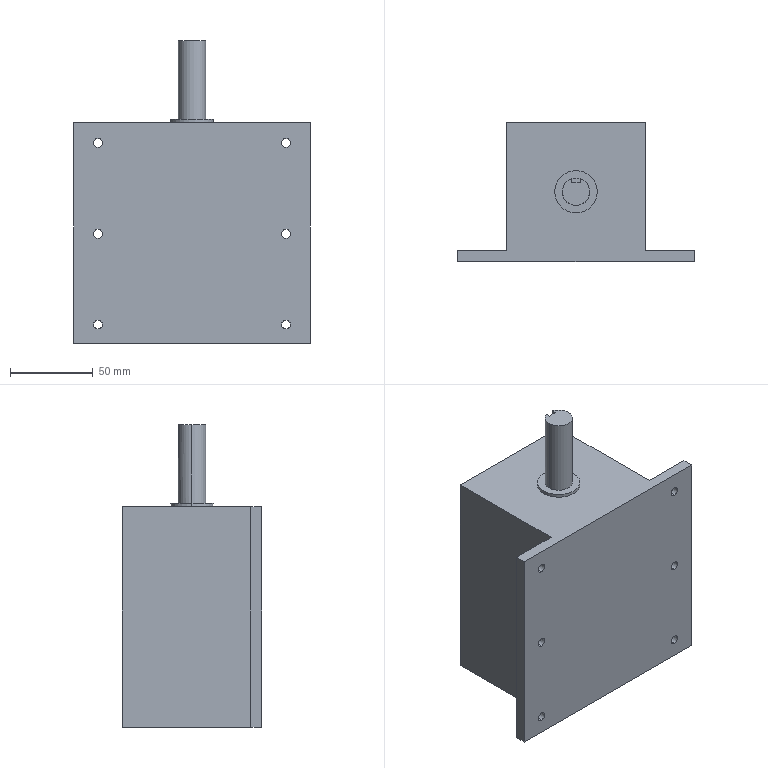Part | SolidWorks | features BaseBody 1, ICE 1 | 1 solid | 32 faces | box 143.331 x 84.235 x 183.45 mm | volume 1010969 mm3 | cylinder 16 | plane 16 | commonest cylinder face diameters 5.365 x12 16.643 x2 25.738 x2
STEP:
#1=CARTESIAN_POINT('',(-135.383,-355.58,-9.625));
#2=VERTEX_POINT('',#1);
#3=CARTESIAN_POINT('',(-135.383,-355.58,-14.99));
#4=VERTEX_POINT('',#3);
#5=CARTESIAN_POINT('',(-135.383,-355.58,-12.308));
#6=DIRECTION('',(0.,-1.,0.));
#7=DIRECTION('',(0.,0.,-1.));
#8=AXIS2_PLACEMENT_3D('',#5,#6,#7);
#9=CIRCLE('',#8,2.683);
#10=EDGE_CURVE('',#2,#4,#9,.T.);
#11=ORIENTED_EDGE('',*,*,#10,.F.);
#12=CARTESIAN_POINT('',(-135.383,-362.11,-9.625));
#13=VERTEX_POINT('',#12);
#14=CARTESIAN_POINT('',(-135.383,-355.58,-9.625));
#15=DIRECTION('',(0.,-1.,0.));
#16=VECTOR('',#15,1000.);
#17=LINE('',#14,#16);
#18=EDGE_CURVE('',#2,#13,#17,.T.);
#19=ORIENTED_EDGE('',*,*,#18,.T.);
#20=CARTESIAN_POINT('',(-135.383,-362.11,-14.99));
#21=VERTEX_POINT('',#20);
#22=CARTESIAN_POINT('',(-135.383,-362.11,-12.308));
#23=DIRECTION('',(0.,1.,0.));
#24=DIRECTION('',(0.,0.,-1.));
#25=AXIS2_PLACEMENT_3D('',#22,#23,#24);
#26=CIRCLE('',#25,2.683);
#27=EDGE_CURVE('',#21,#13,#26,.T.);
#28=ORIENTED_EDGE('',*,*,#27,.F.);
#29=CARTESIAN_POINT('',(-135.383,-355.58,-14.99));
#30=DIRECTION('',(0.,-1.,0.));
#31=VECTOR('',#30,1000.);
#32=LINE('',#29,#31);
#33=EDGE_CURVE('',#4,#21,#32,.T.);
#34=ORIENTED_EDGE('',*,*,#33,.F.);
#35=EDGE_LOOP('',(#11,#19,#28,#34));
#36=FACE_OUTER_BOUND('',#35,.T.);
#37=CARTESIAN_POINT('',(-135.383,-355.58,-12.308));
#38=DIRECTION('',(0.,-1.,0.));
#39=DIRECTION('',(0.,0.,-1.));
#40=AXIS2_PLACEMENT_3D('',#37,#38,#39);
#41=CYLINDRICAL_SURFACE('',#40,2.683);
#42=ADVANCED_FACE('',(#36),#41,.F.);
#43=CARTESIAN_POINT('',(-135.383,-355.58,-64.625));
#44=VERTEX_POINT('',#43);
#45=CARTESIAN_POINT('',(-135.383,-355.58,-69.99));
#46=VERTEX_POINT('',#45);
#47=CARTESIAN_POINT('',(-135.383,-355.58,-67.308));
#48=DIRECTION('',(0.,-1.,0.));
#49=DIRECTION('',(0.,0.,-1.));
#50=AXIS2_PLACEMENT_3D('',#47,#48,#49);
#51=CIRCLE('',#50,2.683);
#52=EDGE_CURVE('',#44,#46,#51,.T.);
#53=ORIENTED_EDGE('',*,*,#52,.F.);
#54=CARTESIAN_POINT('',(-135.383,-362.11,-64.625));
#55=VERTEX_POINT('',#54);
#56=CARTESIAN_POINT('',(-135.383,-355.58,-64.625));
#57=DIRECTION('',(0.,-1.,0.));
#58=VECTOR('',#57,1000.);
#59=LINE('',#56,#58);
#60=EDGE_CURVE('',#44,#55,#59,.T.);
#61=ORIENTED_EDGE('',*,*,#60,.T.);
#62=CARTESIAN_POINT('',(-135.383,-362.11,-69.99));
#63=VERTEX_POINT('',#62);
#64=CARTESIAN_POINT('',(-135.383,-362.11,-67.308));
#65=DIRECTION('',(0.,1.,0.));
#66=DIRECTION('',(0.,0.,-1.));
#67=AXIS2_PLACEMENT_3D('',#64,#65,#66);
#68=CIRCLE('',#67,2.683);
#69=EDGE_CURVE('',#63,#55,#68,.T.);
#70=ORIENTED_EDGE('',*,*,#69,.F.);
#71=CARTESIAN_POINT('',(-135.383,-355.58,-69.99));
#72=DIRECTION('',(0.,-1.,0.));
#73=VECTOR('',#72,1000.);
#74=LINE('',#71,#73);
#75=EDGE_CURVE('',#46,#63,#74,.T.);
#76=ORIENTED_EDGE('',*,*,#75,.F.);
#77=EDGE_LOOP('',(#53,#61,#70,#76));
#78=FACE_OUTER_BOUND('',#77,.T.);
#79=CARTESIAN_POINT('',(-135.383,-355.58,-67.308));
#80=DIRECTION('',(0.,-1.,0.));
#81=DIRECTION('',(0.,0.,-1.));
#82=AXIS2_PLACEMENT_3D('',#79,#80,#81);
#83=CYLINDRICAL_SURFACE('',#82,2.683);
#84=ADVANCED_FACE('',(#78),#83,.F.);
#85=CARTESIAN_POINT('',(-135.383,-355.58,-119.625));
#86=VERTEX_POINT('',#85);
#87=CARTESIAN_POINT('',(-135.383,-355.58,-124.99));
#88=VERTEX_POINT('',#87);
#89=CARTESIAN_POINT('',(-135.383,-355.58,-122.308));
#90=DIRECTION('',(0.,-1.,0.));
#91=DIRECTION('',(0.,0.,-1.));
#92=AXIS2_PLACEMENT_3D('',#89,#90,#91);
#93=CIRCLE('',#92,2.683);
#94=EDGE_CURVE('',#86,#88,#93,.T.);
#95=ORIENTED_EDGE('',*,*,#94,.F.);
#96=CARTESIAN_POINT('',(-135.383,-362.11,-119.625));
#97=VERTEX_POINT('',#96);
#98=CARTESIAN_POINT('',(-135.383,-355.58,-119.625));
#99=DIRECTION('',(0.,-1.,0.));
#100=VECTOR('',#99,1000.);
#101=LINE('',#98,#100);
#102=EDGE_CURVE('',#86,#97,#101,.T.);
#103=ORIENTED_EDGE('',*,*,#102,.T.);
#104=CARTESIAN_POINT('',(-135.383,-362.11,-124.99));
#105=VERTEX_POINT('',#104);
#106=CARTESIAN_POINT('',(-135.383,-362.11,-122.308));
#107=DIRECTION('',(0.,1.,0.));
#108=DIRECTION('',(0.,0.,-1.));
#109=AXIS2_PLACEMENT_3D('',#106,#107,#108);
#110=CIRCLE('',#109,2.683);
#111=EDGE_CURVE('',#105,#97,#110,.T.);
#112=ORIENTED_EDGE('',*,*,#111,.F.);
#113=CARTESIAN_POINT('',(-135.383,-355.58,-124.99));
#114=DIRECTION('',(0.,-1.,0.));
#115=VECTOR('',#114,1000.);
#116=LINE('',#113,#115);
#117=EDGE_CURVE('',#88,#105,#116,.T.);
#118=ORIENTED_EDGE('',*,*,#117,.F.);
#119=EDGE_LOOP('',(#95,#103,#112,#118));
#120=FACE_OUTER_BOUND('',#119,.T.);
#121=CARTESIAN_POINT('',(-135.383,-355.58,-122.308));
#122=DIRECTION('',(0.,-1.,0.));
#123=DIRECTION('',(0.,0.,-1.));
#124=AXIS2_PLACEMENT_3D('',#121,#122,#123);
#125=CYLINDRICAL_SURFACE('',#124,2.683);
#126=ADVANCED_FACE('',(#120),#125,.F.);
#127=CARTESIAN_POINT('',(-21.6,-355.58,-9.625));
#128=VERTEX_POINT('',#127);
#129=CARTESIAN_POINT('',(-21.6,-355.58,-14.99));
#130=VERTEX_POINT('',#129);
#131=CARTESIAN_POINT('',(-21.6,-355.58,-12.308));
#132=DIRECTION('',(0.,-1.,0.));
#133=DIRECTION('',(0.,0.,-1.));
#134=AXIS2_PLACEMENT_3D('',#131,#132,#133);
#135=CIRCLE('',#134,2.683);
#136=EDGE_CURVE('',#128,#130,#135,.T.);
#137=ORIENTED_EDGE('',*,*,#136,.F.);
#138=CARTESIAN_POINT('',(-21.6,-362.11,-9.625));
#139=VERTEX_POINT('',#138);
#140=CARTESIAN_POINT('',(-21.6,-355.58,-9.625));
#141=DIRECTION('',(0.,-1.,0.));
#142=VECTOR('',#141,1000.);
#143=LINE('',#140,#142);
#144=EDGE_CURVE('',#128,#139,#143,.T.);
#145=ORIENTED_EDGE('',*,*,#144,.T.);
#146=CARTESIAN_POINT('',(-21.6,-362.11,-14.99));
#147=VERTEX_POINT('',#146);
#148=CARTESIAN_POINT('',(-21.6,-362.11,-12.308));
#149=DIRECTION('',(0.,1.,0.));
#150=DIRECTION('',(0.,0.,-1.));
#151=AXIS2_PLACEMENT_3D('',#148,#149,#150);
#152=CIRCLE('',#151,2.683);
#153=EDGE_CURVE('',#147,#139,#152,.T.);
#154=ORIENTED_EDGE('',*,*,#153,.F.);
#155=CARTESIAN_POINT('',(-21.6,-355.58,-14.99));
#156=DIRECTION('',(0.,-1.,0.));
#157=VECTOR('',#156,1000.);
#158=LINE('',#155,#157);
#159=EDGE_CURVE('',#130,#147,#158,.T.);
#160=ORIENTED_EDGE('',*,*,#159,.F.);
#161=EDGE_LOOP('',(#137,#145,#154,#160));
#162=FACE_OUTER_BOUND('',#161,.T.);
#163=CARTESIAN_POINT('',(-21.6,-355.58,-12.308));
#164=DIRECTION('',(0.,-1.,0.));
#165=DIRECTION('',(0.,0.,-1.));
#166=AXIS2_PLACEMENT_3D('',#163,#164,#165);
#167=CYLINDRICAL_SURFACE('',#166,2.683);
#168=ADVANCED_FACE('',(#162),#167,.F.);
#169=CARTESIAN_POINT('',(-21.6,-355.58,-64.625));
#170=VERTEX_POINT('',#169);
#171=CARTESIAN_POINT('',(-21.6,-355.58,-69.99));
#172=VERTEX_POINT('',#171);
#173=CARTESIAN_POINT('',(-21.6,-355.58,-67.308));
#174=DIRECTION('',(0.,-1.,0.));
#175=DIRECTION('',(0.,0.,-1.));
#176=AXIS2_PLACEMENT_3D('',#173,#174,#175);
#177=CIRCLE('',#176,2.683);
#178=EDGE_CURVE('',#170,#172,#177,.T.);
#179=ORIENTED_EDGE('',*,*,#178,.F.);
#180=CARTESIAN_POINT('',(-21.6,-362.11,-64.625));
#181=VERTEX_POINT('',#180);
#182=CARTESIAN_POINT('',(-21.6,-355.58,-64.625));
#183=DIRECTION('',(0.,-1.,0.));
#184=VECTOR('',#183,1000.);
#185=LINE('',#182,#184);
#186=EDGE_CURVE('',#170,#181,#185,.T.);
#187=ORIENTED_EDGE('',*,*,#186,.T.);
#188=CARTESIAN_POINT('',(-21.6,-362.11,-69.99));
#189=VERTEX_POINT('',#188);
#190=CARTESIAN_POINT('',(-21.6,-362.11,-67.308));
#191=DIRECTION('',(0.,1.,0.));
#192=DIRECTION('',(0.,0.,-1.));
#193=AXIS2_PLACEMENT_3D('',#190,#191,#192);
#194=CIRCLE('',#193,2.683);
#195=EDGE_CURVE('',#189,#181,#194,.T.);
#196=ORIENTED_EDGE('',*,*,#195,.F.);
#197=CARTESIAN_POINT('',(-21.6,-355.58,-69.99));
#198=DIRECTION('',(0.,-1.,0.));
#199=VECTOR('',#198,1000.);
#200=LINE('',#197,#199);
#201=EDGE_CURVE('',#172,#189,#200,.T.);
#202=ORIENTED_EDGE('',*,*,#201,.F.);
#203=EDGE_LOOP('',(#179,#187,#196,#202));
#204=FACE_OUTER_BOUND('',#203,.T.);
#205=CARTESIAN_POINT('',(-21.6,-355.58,-67.308));
#206=DIRECTION('',(0.,-1.,0.));
#207=DIRECTION('',(0.,0.,-1.));
#208=AXIS2_PLACEMENT_3D('',#205,#206,#207);
#209=CYLINDRICAL_SURFACE('',#208,2.683);
#210=ADVANCED_FACE('',(#204),#209,.F.);
#211=CARTESIAN_POINT('',(-21.6,-355.58,-119.625));
#212=VERTEX_POINT('',#211);
#213=CARTESIAN_POINT('',(-21.6,-355.58,-124.99));
#214=VERTEX_POINT('',#213);
#215=CARTESIAN_POINT('',(-21.6,-355.58,-122.308));
#216=DIRECTION('',(0.,-1.,0.));
#217=DIRECTION('',(0.,0.,-1.));
#218=AXIS2_PLACEMENT_3D('',#215,#216,#217);
#219=CIRCLE('',#218,2.683);
#220=EDGE_CURVE('',#212,#214,#219,.T.);
#221=ORIENTED_EDGE('',*,*,#220,.F.);
#222=CARTESIAN_POINT('',(-21.6,-362.11,-119.625));
#223=VERTEX_POINT('',#222);
#224=CARTESIAN_POINT('',(-21.6,-355.58,-119.625));
#225=DIRECTION('',(0.,-1.,0.));
#226=VECTOR('',#225,1000.);
#227=LINE('',#224,#226);
#228=EDGE_CURVE('',#212,#223,#227,.T.);
#229=ORIENTED_EDGE('',*,*,#228,.T.);
#230=CARTESIAN_POINT('',(-21.6,-362.11,-124.99));
#231=VERTEX_POINT('',#230);
#232=CARTESIAN_POINT('',(-21.6,-362.11,-122.308));
#233=DIRECTION('',(0.,1.,0.));
#234=DIRECTION('',(0.,0.,-1.));
#235=AXIS2_PLACEMENT_3D('',#232,#233,#234);
#236=CIRCLE('',#235,2.683);
#237=EDGE_CURVE('',#231,#223,#236,.T.);
#238=ORIENTED_EDGE('',*,*,#237,.F.);
#239=CARTESIAN_POINT('',(-21.6,-355.58,-124.99));
#240=DIRECTION('',(0.,-1.,0.));
#241=VECTOR('',#240,1000.);
#242=LINE('',#239,#241);
#243=EDGE_CURVE('',#214,#231,#242,.T.);
#244=ORIENTED_EDGE('',*,*,#243,.F.);
#245=EDGE_LOOP('',(#221,#229,#238,#244));
#246=FACE_OUTER_BOUND('',#245,.T.);
#247=CARTESIAN_POINT('',(-21.6,-355.58,-122.308));
#248=DIRECTION('',(0.,-1.,0.));
#249=DIRECTION('',(0.,0.,-1.));
#250=AXIS2_PLACEMENT_3D('',#247,#248,#249);
#251=CYLINDRICAL_SURFACE('',#250,2.683);
#252=ADVANCED_FACE('',(#246),#251,.F.);
#253=CARTESIAN_POINT('',(-65.623,-319.993,0.));
#254=VERTEX_POINT('',#253);
#255=CARTESIAN_POINT('',(-91.361,-319.993,0.));
#256=VERTEX_POINT('',#255);
#257=CARTESIAN_POINT('',(-78.492,-319.993,0.));
#258=DIRECTION('',(0.,0.,1.));
#259=DIRECTION('',(1.,0.,0.));
#260=AXIS2_PLACEMENT_3D('',#257,#258,#259);
#261=CIRCLE('',#260,12.869);
#262=EDGE_CURVE('',#254,#256,#261,.T.);
#263=ORIENTED_EDGE('',*,*,#262,.T.);
#264=CARTESIAN_POINT('',(-91.361,-319.993,2.));
#265=VERTEX_POINT('',#264);
#266=CARTESIAN_POINT('',(-91.361,-319.993,0.));
#267=DIRECTION('',(0.,0.,1.));
#268=VECTOR('',#267,1000.);
#269=LINE('',#266,#268);
#270=EDGE_CURVE('',#256,#265,#269,.T.);
#271=ORIENTED_EDGE('',*,*,#270,.T.);
#272=CARTESIAN_POINT('',(-65.623,-319.993,2.));
#273=VERTEX_POINT('',#272);
#274=CARTESIAN_POINT('',(-78.492,-319.993,2.));
#275=DIRECTION('',(0.,0.,-1.));
#276=DIRECTION('',(1.,0.,0.));
#277=AXIS2_PLACEMENT_3D('',#274,#275,#276);
#278=CIRCLE('',#277,12.869);
#279=EDGE_CURVE('',#265,#273,#278,.T.);
#280=ORIENTED_EDGE('',*,*,#279,.T.);
#281=CARTESIAN_POINT('',(-65.623,-319.993,0.));
#282=DIRECTION('',(0.,0.,1.));
#283=VECTOR('',#282,1000.);
#284=LINE('',#281,#283);
#285=EDGE_CURVE('',#254,#273,#284,.T.);
#286=ORIENTED_EDGE('',*,*,#285,.F.);
#287=EDGE_LOOP('',(#263,#271,#280,#286));
#288=FACE_OUTER_BOUND('',#287,.T.);
#289=CARTESIAN_POINT('',(-78.492,-319.993,0.));
#290=DIRECTION('',(0.,0.,1.));
#291=DIRECTION('',(1.,0.,0.));
#292=AXIS2_PLACEMENT_3D('',#289,#290,#291);
#293=CYLINDRICAL_SURFACE('',#292,12.869);
#294=ADVANCED_FACE('',(#288),#293,.T.);
#295=CARTESIAN_POINT('',(-70.17,-319.993,2.));
#296=VERTEX_POINT('',#295);
#297=CARTESIAN_POINT('',(-86.814,-319.993,2.));
#298=VERTEX_POINT('',#297);
#299=CARTESIAN_POINT('',(-78.492,-319.993,2.));
#300=DIRECTION('',(0.,0.,1.));
#301=DIRECTION('',(1.,0.,0.));
#302=AXIS2_PLACEMENT_3D('',#299,#300,#301);
#303=CIRCLE('',#302,8.322);
#304=EDGE_CURVE('',#296,#298,#303,.T.);
#305=ORIENTED_EDGE('',*,*,#304,.T.);
#306=CARTESIAN_POINT('',(-86.814,-319.993,49.688));
#307=VERTEX_POINT('',#306);
#308=CARTESIAN_POINT('',(-86.814,-319.993,0.));
#309=DIRECTION('',(0.,0.,1.));
#310=VECTOR('',#309,1000.);
#311=LINE('',#308,#310);
#312=EDGE_CURVE('',#298,#307,#311,.T.);
#313=ORIENTED_EDGE('',*,*,#312,.T.);
#314=CARTESIAN_POINT('',(-80.992,-312.055,49.688));
#315=VERTEX_POINT('',#314);
#316=CARTESIAN_POINT('',(-78.492,-319.993,49.688));
#317=DIRECTION('',(0.,0.,-1.));
#318=DIRECTION('',(1.,0.,0.));
#319=AXIS2_PLACEMENT_3D('',#316,#317,#318);
#320=CIRCLE('',#319,8.322);
#321=EDGE_CURVE('',#307,#315,#320,.T.);
#322=ORIENTED_EDGE('',*,*,#321,.T.);
#323=CARTESIAN_POINT('',(-80.992,-312.055,29.688));
#324=VERTEX_POINT('',#323);
#325=CARTESIAN_POINT('',(-80.992,-312.055,0.));
#326=DIRECTION('',(0.,0.,1.));
#327=VECTOR('',#326,1000.);
#328=LINE('',#325,#327);
#329=EDGE_CURVE('',#324,#315,#328,.T.);
#330=ORIENTED_EDGE('',*,*,#329,.F.);
#331=CARTESIAN_POINT('',(-75.992,-312.055,29.688));
#332=VERTEX_POINT('',#331);
#333=CARTESIAN_POINT('',(-78.492,-319.993,29.688));
#334=DIRECTION('',(0.,0.,-1.));
#335=DIRECTION('',(1.,0.,0.));
#336=AXIS2_PLACEMENT_3D('',#333,#334,#335);
#337=CIRCLE('',#336,8.322);
#338=EDGE_CURVE('',#324,#332,#337,.T.);
#339=ORIENTED_EDGE('',*,*,#338,.T.);
#340=CARTESIAN_POINT('',(-75.992,-312.055,49.688));
#341=VERTEX_POINT('',#340);
#342=CARTESIAN_POINT('',(-75.992,-312.055,0.));
#343=DIRECTION('',(0.,0.,-1.));
#344=VECTOR('',#343,1000.);
#345=LINE('',#342,#344);
#346=EDGE_CURVE('',#341,#332,#345,.T.);
#347=ORIENTED_EDGE('',*,*,#346,.F.);
#348=CARTESIAN_POINT('',(-70.17,-319.993,49.688));
#349=VERTEX_POINT('',#348);
#350=CARTESIAN_POINT('',(-78.492,-319.993,49.688));
#351=DIRECTION('',(0.,0.,-1.));
#352=DIRECTION('',(1.,0.,0.));
#353=AXIS2_PLACEMENT_3D('',#350,#351,#352);
#354=CIRCLE('',#353,8.322);
#355=EDGE_CURVE('',#341,#349,#354,.T.);
#356=ORIENTED_EDGE('',*,*,#355,.T.);
#357=CARTESIAN_POINT('',(-70.17,-319.993,0.));
#358=DIRECTION('',(0.,0.,1.));
#359=VECTOR('',#358,1000.);
#360=LINE('',#357,#359);
#361=EDGE_CURVE('',#296,#349,#360,.T.);
#362=ORIENTED_EDGE('',*,*,#361,.F.);
#363=EDGE_LOOP('',(#305,#313,#322,#330,#339,#347,#356,#362));
#364=FACE_OUTER_BOUND('',#363,.T.);
#365=CARTESIAN_POINT('',(-78.492,-319.993,0.));
#366=DIRECTION('',(0.,0.,1.));
#367=DIRECTION('',(1.,0.,0.));
#368=AXIS2_PLACEMENT_3D('',#365,#366,#367);
#369=CYLINDRICAL_SURFACE('',#368,8.322);
#370=ADVANCED_FACE('',(#364),#369,.T.);
#371=ORIENTED_EDGE('',*,*,#27,.T.);
#372=CARTESIAN_POINT('',(-135.383,-362.11,-12.308));
#373=DIRECTION('',(0.,1.,0.));
#374=DIRECTION('',(0.,0.,-1.));
#375=AXIS2_PLACEMENT_3D('',#372,#373,#374);
#376=CIRCLE('',#375,2.683);
#377=EDGE_CURVE('',#13,#21,#376,.T.);
#378=ORIENTED_EDGE('',*,*,#377,.T.);
#379=EDGE_LOOP('',(#371,#378));
#380=FACE_BOUND('',#379,.T.);
#381=ORIENTED_EDGE('',*,*,#69,.T.);
#382=CARTESIAN_POINT('',(-135.383,-362.11,-67.308));
#383=DIRECTION('',(0.,1.,0.));
#384=DIRECTION('',(0.,0.,-1.));
#385=AXIS2_PLACEMENT_3D('',#382,#383,#384);
#386=CIRCLE('',#385,2.683);
#387=EDGE_CURVE('',#55,#63,#386,.T.);
#388=ORIENTED_EDGE('',*,*,#387,.T.);
#389=EDGE_LOOP('',(#381,#388));
#390=FACE_BOUND('',#389,.T.);
#391=ORIENTED_EDGE('',*,*,#111,.T.);
#392=CARTESIAN_POINT('',(-135.383,-362.11,-122.308));
#393=DIRECTION('',(0.,1.,0.));
#394=DIRECTION('',(0.,0.,-1.));
#395=AXIS2_PLACEMENT_3D('',#392,#393,#394);
#396=CIRCLE('',#395,2.683);
#397=EDGE_CURVE('',#97,#105,#396,.T.);
#398=ORIENTED_EDGE('',*,*,#397,.T.);
#399=EDGE_LOOP('',(#391,#398));
#400=FACE_BOUND('',#399,.T.);
#401=ORIENTED_EDGE('',*,*,#153,.T.);
#402=CARTESIAN_POINT('',(-21.6,-362.11,-12.308));
#403=DIRECTION('',(0.,1.,0.));
#404=DIRECTION('',(0.,0.,-1.));
#405=AXIS2_PLACEMENT_3D('',#402,#403,#404);
#406=CIRCLE('',#405,2.683);
#407=EDGE_CURVE('',#139,#147,#406,.T.);
#408=ORIENTED_EDGE('',*,*,#407,.T.);
#409=EDGE_LOOP('',(#401,#408));
#410=FACE_BOUND('',#409,.T.);
#411=ORIENTED_EDGE('',*,*,#195,.T.);
#412=CARTESIAN_POINT('',(-21.6,-362.11,-67.308));
#413=DIRECTION('',(0.,1.,0.));
#414=DIRECTION('',(0.,0.,-1.));
#415=AXIS2_PLACEMENT_3D('',#412,#413,#414);
#416=CIRCLE('',#415,2.683);
#417=EDGE_CURVE('',#181,#189,#416,.T.);
#418=ORIENTED_EDGE('',*,*,#417,.T.);
#419=EDGE_LOOP('',(#411,#418));
#420=FACE_BOUND('',#419,.T.);
#421=ORIENTED_EDGE('',*,*,#237,.T.);
#422=CARTESIAN_POINT('',(-21.6,-362.11,-122.308));
#423=DIRECTION('',(0.,1.,0.));
#424=DIRECTION('',(0.,0.,-1.));
#425=AXIS2_PLACEMENT_3D('',#422,#423,#424);
#426=CIRCLE('',#425,2.683);
#427=EDGE_CURVE('',#223,#231,#426,.T.);
#428=ORIENTED_EDGE('',*,*,#427,.T.);
#429=EDGE_LOOP('',(#421,#428));
#430=FACE_BOUND('',#429,.T.);
#431=CARTESIAN_POINT('',(-150.157,-362.11,-133.762));
#432=VERTEX_POINT('',#431);
#433=CARTESIAN_POINT('',(-6.826,-362.11,-133.762));
#434=VERTEX_POINT('',#433);
#435=CARTESIAN_POINT('',(-6.826,-362.11,-133.762));
#436=DIRECTION('',(1.,0.,0.));
#437=VECTOR('',#436,1000.);
#438=LINE('',#435,#437);
#439=EDGE_CURVE('',#432,#434,#438,.T.);
#440=ORIENTED_EDGE('',*,*,#439,.T.);
#441=CARTESIAN_POINT('',(-6.826,-362.11,0.));
#442=VERTEX_POINT('',#441);
#443=CARTESIAN_POINT('',(-6.826,-362.11,0.));
#444=DIRECTION('',(0.,0.,1.));
#445=VECTOR('',#444,1000.);
#446=LINE('',#443,#445);
#447=EDGE_CURVE('',#434,#442,#446,.T.);
#448=ORIENTED_EDGE('',*,*,#447,.T.);
#449=CARTESIAN_POINT('',(-150.157,-362.11,0.));
#450=VERTEX_POINT('',#449);
#451=CARTESIAN_POINT('',(-6.826,-362.11,0.));
#452=DIRECTION('',(-1.,0.,0.));
#453=VECTOR('',#452,1000.);
#454=LINE('',#451,#453);
#455=EDGE_CURVE('',#442,#450,#454,.T.);
#456=ORIENTED_EDGE('',*,*,#455,.T.);
#457=CARTESIAN_POINT('',(-150.157,-362.11,0.));
#458=DIRECTION('',(0.,0.,-1.));
#459=VECTOR('',#458,1000.);
#460=LINE('',#457,#459);
#461=EDGE_CURVE('',#450,#432,#460,.T.);
#462=ORIENTED_EDGE('',*,*,#461,.T.);
#463=EDGE_LOOP('',(#440,#448,#456,#462));
#464=FACE_OUTER_BOUND('',#463,.T.);
#465=CARTESIAN_POINT('',(-6.826,-362.11,0.));
#466=DIRECTION('',(0.,-1.,0.));
#467=DIRECTION('',(0.,0.,-1.));
#468=AXIS2_PLACEMENT_3D('',#465,#466,#467);
#469=PLANE('',#468);
#470=ADVANCED_FACE('',(#380,#390,#400,#410,#420,#430,#464),#469,.T.);
#471=ORIENTED_EDGE('',*,*,#18,.F.);
#472=CARTESIAN_POINT('',(-135.383,-355.58,-12.308));
#473=DIRECTION('',(0.,-1.,0.));
#474=DIRECTION('',(0.,0.,-1.));
#475=AXIS2_PLACEMENT_3D('',#472,#473,#474);
#476=CIRCLE('',#475,2.683);
#477=EDGE_CURVE('',#4,#2,#476,.T.);
#478=ORIENTED_EDGE('',*,*,#477,.F.);
#479=ORIENTED_EDGE('',*,*,#33,.T.);
#480=ORIENTED_EDGE('',*,*,#377,.F.);
#481=EDGE_LOOP('',(#471,#478,#479,#480));
#482=FACE_OUTER_BOUND('',#481,.T.);
#483=CARTESIAN_POINT('',(-135.383,-355.58,-12.308));
#484=DIRECTION('',(0.,-1.,0.));
#485=DIRECTION('',(0.,0.,-1.));
#486=AXIS2_PLACEMENT_3D('',#483,#484,#485);
#487=CYLINDRICAL_SURFACE('',#486,2.683);
#488=ADVANCED_FACE('',(#482),#487,.F.);
#489=ORIENTED_EDGE('',*,*,#60,.F.);
#490=CARTESIAN_POINT('',(-135.383,-355.58,-67.308));
#491=DIRECTION('',(0.,-1.,0.));
#492=DIRECTION('',(0.,0.,-1.));
#493=AXIS2_PLACEMENT_3D('',#490,#491,#492);
#494=CIRCLE('',#493,2.683);
#495=EDGE_CURVE('',#46,#44,#494,.T.);
#496=ORIENTED_EDGE('',*,*,#495,.F.);
#497=ORIENTED_EDGE('',*,*,#75,.T.);
#498=ORIENTED_EDGE('',*,*,#387,.F.);
#499=EDGE_LOOP('',(#489,#496,#497,#498));
#500=FACE_OUTER_BOUND('',#499,.T.);
#501=CARTESIAN_POINT('',(-135.383,-355.58,-67.308));
#502=DIRECTION('',(0.,-1.,0.));
#503=DIRECTION('',(0.,0.,-1.));
#504=AXIS2_PLACEMENT_3D('',#501,#502,#503);
#505=CYLINDRICAL_SURFACE('',#504,2.683);
#506=ADVANCED_FACE('',(#500),#505,.F.);
#507=ORIENTED_EDGE('',*,*,#102,.F.);
#508=CARTESIAN_POINT('',(-135.383,-355.58,-122.308));
#509=DIRECTION('',(0.,-1.,0.));
#510=DIRECTION('',(0.,0.,-1.));
#511=AXIS2_PLACEMENT_3D('',#508,#509,#510);
#512=CIRCLE('',#511,2.683);
#513=EDGE_CURVE('',#88,#86,#512,.T.);
#514=ORIENTED_EDGE('',*,*,#513,.F.);
#515=ORIENTED_EDGE('',*,*,#117,.T.);
#516=ORIENTED_EDGE('',*,*,#397,.F.);
#517=EDGE_LOOP('',(#507,#514,#515,#516));
#518=FACE_OUTER_BOUND('',#517,.T.);
#519=CARTESIAN_POINT('',(-135.383,-355.58,-122.308));
#520=DIRECTION('',(0.,-1.,0.));
#521=DIRECTION('',(0.,0.,-1.));
#522=AXIS2_PLACEMENT_3D('',#519,#520,#521);
#523=CYLINDRICAL_SURFACE('',#522,2.683);
#524=ADVANCED_FACE('',(#518),#523,.F.);
#525=ORIENTED_EDGE('',*,*,#144,.F.);
#526=CARTESIAN_POINT('',(-21.6,-355.58,-12.308));
#527=DIRECTION('',(0.,-1.,0.));
#528=DIRECTION('',(0.,0.,-1.));
#529=AXIS2_PLACEMENT_3D('',#526,#527,#528);
#530=CIRCLE('',#529,2.683);
#531=EDGE_CURVE('',#130,#128,#530,.T.);
#532=ORIENTED_EDGE('',*,*,#531,.F.);
#533=ORIENTED_EDGE('',*,*,#159,.T.);
#534=ORIENTED_EDGE('',*,*,#407,.F.);
#535=EDGE_LOOP('',(#525,#532,#533,#534));
#536=FACE_OUTER_BOUND('',#535,.T.);
#537=CARTESIAN_POINT('',(-21.6,-355.58,-12.308));
#538=DIRECTION('',(0.,-1.,0.));
#539=DIRECTION('',(0.,0.,-1.));
#540=AXIS2_PLACEMENT_3D('',#537,#538,#539);
#541=CYLINDRICAL_SURFACE('',#540,2.683);
#542=ADVANCED_FACE('',(#536),#541,.F.);
#543=ORIENTED_EDGE('',*,*,#186,.F.);
#544=CARTESIAN_POINT('',(-21.6,-355.58,-67.308));
#545=DIRECTION('',(0.,-1.,0.));
#546=DIRECTION('',(0.,0.,-1.));
#547=AXIS2_PLACEMENT_3D('',#544,#545,#546);
#548=CIRCLE('',#547,2.683);
#549=EDGE_CURVE('',#172,#170,#548,.T.);
#550=ORIENTED_EDGE('',*,*,#549,.F.);
#551=ORIENTED_EDGE('',*,*,#201,.T.);
#552=ORIENTED_EDGE('',*,*,#417,.F.);
#553=EDGE_LOOP('',(#543,#550,#551,#552));
#554=FACE_OUTER_BOUND('',#553,.T.);
#555=CARTESIAN_POINT('',(-21.6,-355.58,-67.308));
#556=DIRECTION('',(0.,-1.,0.));
#557=DIRECTION('',(0.,0.,-1.));
#558=AXIS2_PLACEMENT_3D('',#555,#556,#557);
#559=CYLINDRICAL_SURFACE('',#558,2.683);
#560=ADVANCED_FACE('',(#554),#559,.F.);
#561=ORIENTED_EDGE('',*,*,#228,.F.);
#562=CARTESIAN_POINT('',(-21.6,-355.58,-122.308));
#563=DIRECTION('',(0.,-1.,0.));
#564=DIRECTION('',(0.,0.,-1.));
#565=AXIS2_PLACEMENT_3D('',#562,#563,#564);
#566=CIRCLE('',#565,2.683);
#567=EDGE_CURVE('',#214,#212,#566,.T.);
#568=ORIENTED_EDGE('',*,*,#567,.F.);
#569=ORIENTED_EDGE('',*,*,#243,.T.);
#570=ORIENTED_EDGE('',*,*,#427,.F.);
#571=EDGE_LOOP('',(#561,#568,#569,#570));
#572=FACE_OUTER_BOUND('',#571,.T.);
#573=CARTESIAN_POINT('',(-21.6,-355.58,-122.308));
#574=DIRECTION('',(0.,-1.,0.));
#575=DIRECTION('',(0.,0.,-1.));
#576=AXIS2_PLACEMENT_3D('',#573,#574,#575);
#577=CYLINDRICAL_SURFACE('',#576,2.683);
#578=ADVANCED_FACE('',(#572),#577,.F.);
#579=CARTESIAN_POINT('',(-6.826,-355.58,-133.762));
#580=VERTEX_POINT('',#579);
#581=CARTESIAN_POINT('',(-6.826,-355.58,-133.762));
#582=DIRECTION('',(0.,1.,0.));
#583=VECTOR('',#582,1000.);
#584=LINE('',#581,#583);
#585=EDGE_CURVE('',#434,#580,#584,.T.);
#586=ORIENTED_EDGE('',*,*,#585,.T.);
#587=CARTESIAN_POINT('',(-6.826,-355.58,0.));
#588=VERTEX_POINT('',#587);
#589=CARTESIAN_POINT('',(-6.826,-355.58,0.));
#590=DIRECTION('',(0.,0.,1.));
#591=VECTOR('',#590,1000.);
#592=LINE('',#589,#591);
#593=EDGE_CURVE('',#580,#588,#592,.T.);
#594=ORIENTED_EDGE('',*,*,#593,.T.);
#595=CARTESIAN_POINT('',(-6.826,-355.58,0.));
#596=DIRECTION('',(0.,-1.,0.));
#597=VECTOR('',#596,1000.);
#598=LINE('',#595,#597);
#599=EDGE_CURVE('',#588,#442,#598,.T.);
#600=ORIENTED_EDGE('',*,*,#599,.T.);
#601=ORIENTED_EDGE('',*,*,#447,.F.);
#602=EDGE_LOOP('',(#586,#594,#600,#601));
#603=FACE_OUTER_BOUND('',#602,.T.);
#604=CARTESIAN_POINT('',(-6.826,-355.58,0.));
#605=DIRECTION('',(1.,0.,0.));
#606=DIRECTION('',(0.,0.,-1.));
#607=AXIS2_PLACEMENT_3D('',#604,#605,#606);
#608=PLANE('',#607);
#609=ADVANCED_FACE('',(#603),#608,.T.);
#610=CARTESIAN_POINT('',(-120.609,-355.58,-133.762));
#611=VERTEX_POINT('',#610);
#612=CARTESIAN_POINT('',(-120.609,-277.875,-133.762));
#613=VERTEX_POINT('',#612);
#614=CARTESIAN_POINT('',(-120.609,-319.993,-133.762));
#615=DIRECTION('',(0.,1.,0.));
#616=VECTOR('',#615,1000.);
#617=LINE('',#614,#616);
#618=EDGE_CURVE('',#611,#613,#617,.T.);
#619=ORIENTED_EDGE('',*,*,#618,.T.);
#620=CARTESIAN_POINT('',(-36.374,-277.875,-133.762));
#621=VERTEX_POINT('',#620);
#622=CARTESIAN_POINT('',(-78.492,-277.875,-133.762));
#623=DIRECTION('',(1.,0.,0.));
#624=VECTOR('',#623,1000.);
#625=LINE('',#622,#624);
#626=EDGE_CURVE('',#613,#621,#625,.T.);
#627=ORIENTED_EDGE('',*,*,#626,.T.);
#628=CARTESIAN_POINT('',(-36.374,-355.58,-133.762));
#629=VERTEX_POINT('',#628);
#630=CARTESIAN_POINT('',(-36.374,-319.993,-133.762));
#631=DIRECTION('',(0.,-1.,0.));
#632=VECTOR('',#631,1000.);
#633=LINE('',#630,#632);
#634=EDGE_CURVE('',#621,#629,#633,.T.);
#635=ORIENTED_EDGE('',*,*,#634,.T.);
#636=CARTESIAN_POINT('',(-78.492,-355.58,-133.762));
#637=DIRECTION('',(1.,0.,0.));
#638=VECTOR('',#637,1000.);
#639=LINE('',#636,#638);
#640=EDGE_CURVE('',#629,#580,#639,.T.);
#641=ORIENTED_EDGE('',*,*,#640,.T.);
#642=ORIENTED_EDGE('',*,*,#585,.F.);
#643=ORIENTED_EDGE('',*,*,#439,.F.);
#644=CARTESIAN_POINT('',(-150.157,-355.58,-133.762));
#645=VERTEX_POINT('',#644);
#646=CARTESIAN_POINT('',(-150.157,-319.993,-133.762));
#647=DIRECTION('',(0.,1.,0.));
#648=VECTOR('',#647,1000.);
#649=LINE('',#646,#648);
#650=EDGE_CURVE('',#432,#645,#649,.T.);
#651=ORIENTED_EDGE('',*,*,#650,.T.);
#652=CARTESIAN_POINT('',(-78.492,-355.58,-133.762));
#653=DIRECTION('',(1.,0.,0.));
#654=VECTOR('',#653,1000.);
#655=LINE('',#652,#654);
#656=EDGE_CURVE('',#645,#611,#655,.T.);
#657=ORIENTED_EDGE('',*,*,#656,.T.);
#658=EDGE_LOOP('',(#619,#627,#635,#641,#642,#643,#651,#657));
#659=FACE_OUTER_BOUND('',#658,.T.);
#660=CARTESIAN_POINT('',(-78.492,-319.993,-133.762));
#661=DIRECTION('',(0.,0.,-1.));
#662=DIRECTION('',(-1.,0.,0.));
#663=AXIS2_PLACEMENT_3D('',#660,#661,#662);
#664=PLANE('',#663);
#665=ADVANCED_FACE('',(#659),#664,.T.);
#666=ORIENTED_EDGE('',*,*,#650,.F.);
#667=ORIENTED_EDGE('',*,*,#461,.F.);
#668=CARTESIAN_POINT('',(-150.157,-355.58,0.));
#669=VERTEX_POINT('',#668);
#670=CARTESIAN_POINT('',(-150.157,-362.11,0.));
#671=DIRECTION('',(0.,1.,0.));
#672=VECTOR('',#671,1000.);
#673=LINE('',#670,#672);
#674=EDGE_CURVE('',#450,#669,#673,.T.);
#675=ORIENTED_EDGE('',*,*,#674,.T.);
#676=CARTESIAN_POINT('',(-150.157,-355.58,0.));
#677=DIRECTION('',(0.,0.,-1.));
#678=VECTOR('',#677,1000.);
#679=LINE('',#676,#678);
#680=EDGE_CURVE('',#669,#645,#679,.T.);
#681=ORIENTED_EDGE('',*,*,#680,.T.);
#682=EDGE_LOOP('',(#666,#667,#675,#681));
#683=FACE_OUTER_BOUND('',#682,.T.);
#684=CARTESIAN_POINT('',(-150.157,-362.11,0.));
#685=DIRECTION('',(-1.,0.,0.));
#686=DIRECTION('',(0.,0.,1.));
#687=AXIS2_PLACEMENT_3D('',#684,#685,#686);
#688=PLANE('',#687);
#689=ADVANCED_FACE('',(#683),#688,.T.);
#690=ORIENTED_EDGE('',*,*,#262,.F.);
#691=CARTESIAN_POINT('',(-78.492,-319.993,0.));
#692=DIRECTION('',(0.,0.,1.));
#693=DIRECTION('',(1.,0.,0.));
#694=AXIS2_PLACEMENT_3D('',#691,#692,#693);
#695=CIRCLE('',#694,12.869);
#696=EDGE_CURVE('',#256,#254,#695,.T.);
#697=ORIENTED_EDGE('',*,*,#696,.F.);
#698=EDGE_LOOP('',(#690,#697));
#699=FACE_BOUND('',#698,.T.);
#700=CARTESIAN_POINT('',(-120.609,-277.875,0.));
#701=VERTEX_POINT('',#700);
#702=CARTESIAN_POINT('',(-36.374,-277.875,0.));
#703=VERTEX_POINT('',#702);
#704=CARTESIAN_POINT('',(-78.492,-277.875,0.));
#705=DIRECTION('',(1.,0.,0.));
#706=VECTOR('',#705,1000.);
#707=LINE('',#704,#706);
#708=EDGE_CURVE('',#701,#703,#707,.T.);
#709=ORIENTED_EDGE('',*,*,#708,.F.);
#710=CARTESIAN_POINT('',(-120.609,-355.58,0.));
#711=VERTEX_POINT('',#710);
#712=CARTESIAN_POINT('',(-120.609,-319.993,0.));
#713=DIRECTION('',(0.,1.,0.));
#714=VECTOR('',#713,1000.);
#715=LINE('',#712,#714);
#716=EDGE_CURVE('',#711,#701,#715,.T.);
#717=ORIENTED_EDGE('',*,*,#716,.F.);
#718=CARTESIAN_POINT('',(-78.492,-355.58,0.));
#719=DIRECTION('',(1.,0.,0.));
#720=VECTOR('',#719,1000.);
#721=LINE('',#718,#720);
#722=EDGE_CURVE('',#669,#711,#721,.T.);
#723=ORIENTED_EDGE('',*,*,#722,.F.);
#724=ORIENTED_EDGE('',*,*,#674,.F.);
#725=ORIENTED_EDGE('',*,*,#455,.F.);
#726=ORIENTED_EDGE('',*,*,#599,.F.);
#727=CARTESIAN_POINT('',(-36.374,-355.58,0.));
#728=VERTEX_POINT('',#727);
#729=CARTESIAN_POINT('',(-78.492,-355.58,0.));
#730=DIRECTION('',(1.,0.,0.));
#731=VECTOR('',#730,1000.);
#732=LINE('',#729,#731);
#733=EDGE_CURVE('',#728,#588,#732,.T.);
#734=ORIENTED_EDGE('',*,*,#733,.F.);
#735=CARTESIAN_POINT('',(-36.374,-319.993,0.));
#736=DIRECTION('',(0.,-1.,0.));
#737=VECTOR('',#736,1000.);
#738=LINE('',#735,#737);
#739=EDGE_CURVE('',#703,#728,#738,.T.);
#740=ORIENTED_EDGE('',*,*,#739,.F.);
#741=EDGE_LOOP('',(#709,#717,#723,#724,#725,#726,#734,#740));
#742=FACE_OUTER_BOUND('',#741,.T.);
#743=CARTESIAN_POINT('',(-78.492,-319.993,0.));
#744=DIRECTION('',(0.,0.,-1.));
#745=DIRECTION('',(-1.,0.,0.));
#746=AXIS2_PLACEMENT_3D('',#743,#744,#745);
#747=PLANE('',#746);
#748=ADVANCED_FACE('',(#699,#742),#747,.F.);
#749=ORIENTED_EDGE('',*,*,#477,.T.);
#750=ORIENTED_EDGE('',*,*,#10,.T.);
#751=EDGE_LOOP('',(#749,#750));
#752=FACE_BOUND('',#751,.T.);
#753=ORIENTED_EDGE('',*,*,#495,.T.);
#754=ORIENTED_EDGE('',*,*,#52,.T.);
#755=EDGE_LOOP('',(#753,#754));
#756=FACE_BOUND('',#755,.T.);
#757=ORIENTED_EDGE('',*,*,#513,.T.);
#758=ORIENTED_EDGE('',*,*,#94,.T.);
#759=EDGE_LOOP('',(#757,#758));
#760=FACE_BOUND('',#759,.T.);
#761=ORIENTED_EDGE('',*,*,#656,.F.);
#762=ORIENTED_EDGE('',*,*,#680,.F.);
#763=ORIENTED_EDGE('',*,*,#722,.T.);
#764=CARTESIAN_POINT('',(-120.609,-355.58,0.));
#765=DIRECTION('',(0.,0.,-1.));
#766=VECTOR('',#765,1000.);
#767=LINE('',#764,#766);
#768=EDGE_CURVE('',#711,#611,#767,.T.);
#769=ORIENTED_EDGE('',*,*,#768,.T.);
#770=EDGE_LOOP('',(#761,#762,#763,#769));
#771=FACE_OUTER_BOUND('',#770,.T.);
#772=CARTESIAN_POINT('',(-150.157,-355.58,0.));
#773=DIRECTION('',(0.,1.,0.));
#774=DIRECTION('',(0.,0.,1.));
#775=AXIS2_PLACEMENT_3D('',#772,#773,#774);
#776=PLANE('',#775);
#777=ADVANCED_FACE('',(#752,#756,#760,#771),#776,.T.);
#778=ORIENTED_EDGE('',*,*,#531,.T.);
#779=ORIENTED_EDGE('',*,*,#136,.T.);
#780=EDGE_LOOP('',(#778,#779));
#781=FACE_BOUND('',#780,.T.);
#782=ORIENTED_EDGE('',*,*,#549,.T.);
#783=ORIENTED_EDGE('',*,*,#178,.T.);
#784=EDGE_LOOP('',(#782,#783));
#785=FACE_BOUND('',#784,.T.);
#786=ORIENTED_EDGE('',*,*,#567,.T.);
#787=ORIENTED_EDGE('',*,*,#220,.T.);
#788=EDGE_LOOP('',(#786,#787));
#789=FACE_BOUND('',#788,.T.);
#790=ORIENTED_EDGE('',*,*,#640,.F.);
#791=CARTESIAN_POINT('',(-36.374,-355.58,0.));
#792=DIRECTION('',(0.,0.,1.));
#793=VECTOR('',#792,1000.);
#794=LINE('',#791,#793);
#795=EDGE_CURVE('',#629,#728,#794,.T.);
#796=ORIENTED_EDGE('',*,*,#795,.T.);
#797=ORIENTED_EDGE('',*,*,#733,.T.);
#798=ORIENTED_EDGE('',*,*,#593,.F.);
#799=EDGE_LOOP('',(#790,#796,#797,#798));
#800=FACE_OUTER_BOUND('',#799,.T.);
#801=CARTESIAN_POINT('',(-36.374,-355.58,0.));
#802=DIRECTION('',(0.,1.,0.));
#803=DIRECTION('',(0.,0.,1.));
#804=AXIS2_PLACEMENT_3D('',#801,#802,#803);
#805=PLANE('',#804);
#806=ADVANCED_FACE('',(#781,#785,#789,#800),#805,.T.);
#807=ORIENTED_EDGE('',*,*,#626,.F.);
#808=CARTESIAN_POINT('',(-120.609,-277.875,0.));
#809=DIRECTION('',(0.,0.,1.));
#810=VECTOR('',#809,1000.);
#811=LINE('',#808,#810);
#812=EDGE_CURVE('',#613,#701,#811,.T.);
#813=ORIENTED_EDGE('',*,*,#812,.T.);
#814=ORIENTED_EDGE('',*,*,#708,.T.);
#815=CARTESIAN_POINT('',(-36.374,-277.875,0.));
#816=DIRECTION('',(0.,0.,-1.));
#817=VECTOR('',#816,1000.);
#818=LINE('',#815,#817);
#819=EDGE_CURVE('',#703,#621,#818,.T.);
#820=ORIENTED_EDGE('',*,*,#819,.T.);
#821=EDGE_LOOP('',(#807,#813,#814,#820));
#822=FACE_OUTER_BOUND('',#821,.T.);
#823=CARTESIAN_POINT('',(-120.609,-277.875,0.));
#824=DIRECTION('',(0.,1.,0.));
#825=DIRECTION('',(0.,0.,1.));
#826=AXIS2_PLACEMENT_3D('',#823,#824,#825);
#827=PLANE('',#826);
#828=ADVANCED_FACE('',(#822),#827,.T.);
#829=ORIENTED_EDGE('',*,*,#618,.F.);
#830=ORIENTED_EDGE('',*,*,#768,.F.);
#831=ORIENTED_EDGE('',*,*,#716,.T.);
#832=ORIENTED_EDGE('',*,*,#812,.F.);
#833=EDGE_LOOP('',(#829,#830,#831,#832));
#834=FACE_OUTER_BOUND('',#833,.T.);
#835=CARTESIAN_POINT('',(-120.609,-355.58,0.));
#836=DIRECTION('',(-1.,0.,0.));
#837=DIRECTION('',(0.,0.,1.));
#838=AXIS2_PLACEMENT_3D('',#835,#836,#837);
#839=PLANE('',#838);
#840=ADVANCED_FACE('',(#834),#839,.T.);
#841=ORIENTED_EDGE('',*,*,#634,.F.);
#842=ORIENTED_EDGE('',*,*,#819,.F.);
#843=ORIENTED_EDGE('',*,*,#739,.T.);
#844=ORIENTED_EDGE('',*,*,#795,.F.);
#845=EDGE_LOOP('',(#841,#842,#843,#844));
#846=FACE_OUTER_BOUND('',#845,.T.);
#847=CARTESIAN_POINT('',(-36.374,-277.875,0.));
#848=DIRECTION('',(1.,0.,0.));
#849=DIRECTION('',(0.,0.,-1.));
#850=AXIS2_PLACEMENT_3D('',#847,#848,#849);
#851=PLANE('',#850);
#852=ADVANCED_FACE('',(#846),#851,.T.);
#853=ORIENTED_EDGE('',*,*,#270,.F.);
#854=ORIENTED_EDGE('',*,*,#696,.T.);
#855=ORIENTED_EDGE('',*,*,#285,.T.);
#856=CARTESIAN_POINT('',(-78.492,-319.993,2.));
#857=DIRECTION('',(0.,0.,-1.));
#858=DIRECTION('',(1.,0.,0.));
#859=AXIS2_PLACEMENT_3D('',#856,#857,#858);
#860=CIRCLE('',#859,12.869);
#861=EDGE_CURVE('',#273,#265,#860,.T.);
#862=ORIENTED_EDGE('',*,*,#861,.T.);
#863=EDGE_LOOP('',(#853,#854,#855,#862));
#864=FACE_OUTER_BOUND('',#863,.T.);
#865=CARTESIAN_POINT('',(-78.492,-319.993,0.));
#866=DIRECTION('',(0.,0.,1.));
#867=DIRECTION('',(1.,0.,0.));
#868=AXIS2_PLACEMENT_3D('',#865,#866,#867);
#869=CYLINDRICAL_SURFACE('',#868,12.869);
#870=ADVANCED_FACE('',(#864),#869,.T.);
#871=ORIENTED_EDGE('',*,*,#304,.F.);
#872=CARTESIAN_POINT('',(-78.492,-319.993,2.));
#873=DIRECTION('',(0.,0.,1.));
#874=DIRECTION('',(1.,0.,0.));
#875=AXIS2_PLACEMENT_3D('',#872,#873,#874);
#876=CIRCLE('',#875,8.322);
#877=EDGE_CURVE('',#298,#296,#876,.T.);
#878=ORIENTED_EDGE('',*,*,#877,.F.);
#879=EDGE_LOOP('',(#871,#878));
#880=FACE_BOUND('',#879,.T.);
#881=ORIENTED_EDGE('',*,*,#861,.F.);
#882=ORIENTED_EDGE('',*,*,#279,.F.);
#883=EDGE_LOOP('',(#881,#882));
#884=FACE_OUTER_BOUND('',#883,.T.);
#885=CARTESIAN_POINT('',(-78.492,-319.993,2.));
#886=DIRECTION('',(0.,0.,-1.));
#887=DIRECTION('',(-1.,0.,0.));
#888=AXIS2_PLACEMENT_3D('',#885,#886,#887);
#889=PLANE('',#888);
#890=ADVANCED_FACE('',(#880,#884),#889,.F.);
#891=ORIENTED_EDGE('',*,*,#312,.F.);
#892=ORIENTED_EDGE('',*,*,#877,.T.);
#893=ORIENTED_EDGE('',*,*,#361,.T.);
#894=CARTESIAN_POINT('',(-78.492,-319.993,49.688));
#895=DIRECTION('',(0.,0.,-1.));
#896=DIRECTION('',(1.,0.,0.));
#897=AXIS2_PLACEMENT_3D('',#894,#895,#896);
#898=CIRCLE('',#897,8.322);
#899=EDGE_CURVE('',#349,#307,#898,.T.);
#900=ORIENTED_EDGE('',*,*,#899,.T.);
#901=EDGE_LOOP('',(#891,#892,#893,#900));
#902=FACE_OUTER_BOUND('',#901,.T.);
#903=CARTESIAN_POINT('',(-78.492,-319.993,0.));
#904=DIRECTION('',(0.,0.,1.));
#905=DIRECTION('',(1.,0.,0.));
#906=AXIS2_PLACEMENT_3D('',#903,#904,#905);
#907=CYLINDRICAL_SURFACE('',#906,8.322);
#908=ADVANCED_FACE('',(#902),#907,.T.);
#909=CARTESIAN_POINT('',(-80.992,-314.671,49.688));
#910=VERTEX_POINT('',#909);
#911=CARTESIAN_POINT('',(-80.992,-311.671,49.688));
#912=DIRECTION('',(0.,-1.,0.));
#913=VECTOR('',#912,1000.);
#914=LINE('',#911,#913);
#915=EDGE_CURVE('',#315,#910,#914,.T.);
#916=ORIENTED_EDGE('',*,*,#915,.F.);
#917=ORIENTED_EDGE('',*,*,#321,.F.);
#918=ORIENTED_EDGE('',*,*,#899,.F.);
#919=ORIENTED_EDGE('',*,*,#355,.F.);
#920=CARTESIAN_POINT('',(-75.992,-314.671,49.688));
#921=VERTEX_POINT('',#920);
#922=CARTESIAN_POINT('',(-75.992,-311.671,49.688));
#923=DIRECTION('',(0.,1.,0.));
#924=VECTOR('',#923,1000.);
#925=LINE('',#922,#924);
#926=EDGE_CURVE('',#921,#341,#925,.T.);
#927=ORIENTED_EDGE('',*,*,#926,.F.);
#928=CARTESIAN_POINT('',(-80.992,-314.671,49.688));
#929=DIRECTION('',(1.,0.,0.));
#930=VECTOR('',#929,1000.);
#931=LINE('',#928,#930);
#932=EDGE_CURVE('',#910,#921,#931,.T.);
#933=ORIENTED_EDGE('',*,*,#932,.F.);
#934=EDGE_LOOP('',(#916,#917,#918,#919,#927,#933));
#935=FACE_OUTER_BOUND('',#934,.T.);
#936=CARTESIAN_POINT('',(-78.492,-319.993,49.688));
#937=DIRECTION('',(0.,0.,1.));
#938=DIRECTION('',(1.,0.,0.));
#939=AXIS2_PLACEMENT_3D('',#936,#937,#938);
#940=PLANE('',#939);
#941=ADVANCED_FACE('',(#935),#940,.T.);
#942=ORIENTED_EDGE('',*,*,#329,.T.);
#943=ORIENTED_EDGE('',*,*,#915,.T.);
#944=CARTESIAN_POINT('',(-80.992,-314.671,29.688));
#945=VERTEX_POINT('',#944);
#946=CARTESIAN_POINT('',(-80.992,-314.671,29.688));
#947=DIRECTION('',(0.,0.,1.));
#948=VECTOR('',#947,1000.);
#949=LINE('',#946,#948);
#950=EDGE_CURVE('',#945,#910,#949,.T.);
#951=ORIENTED_EDGE('',*,*,#950,.F.);
#952=CARTESIAN_POINT('',(-80.992,-311.671,29.688));
#953=DIRECTION('',(0.,-1.,0.));
#954=VECTOR('',#953,1000.);
#955=LINE('',#952,#954);
#956=EDGE_CURVE('',#324,#945,#955,.T.);
#957=ORIENTED_EDGE('',*,*,#956,.F.);
#958=EDGE_LOOP('',(#942,#943,#951,#957));
#959=FACE_OUTER_BOUND('',#958,.T.);
#960=CARTESIAN_POINT('',(-80.992,-311.671,29.688));
#961=DIRECTION('',(-1.,0.,0.));
#962=DIRECTION('',(0.,0.,1.));
#963=AXIS2_PLACEMENT_3D('',#960,#961,#962);
#964=PLANE('',#963);
#965=ADVANCED_FACE('',(#959),#964,.F.);
#966=ORIENTED_EDGE('',*,*,#346,.T.);
#967=CARTESIAN_POINT('',(-75.992,-314.671,29.688));
#968=VERTEX_POINT('',#967);
#969=CARTESIAN_POINT('',(-75.992,-311.671,29.688));
#970=DIRECTION('',(0.,1.,0.));
#971=VECTOR('',#970,1000.);
#972=LINE('',#969,#971);
#973=EDGE_CURVE('',#968,#332,#972,.T.);
#974=ORIENTED_EDGE('',*,*,#973,.F.);
#975=CARTESIAN_POINT('',(-75.992,-314.671,29.688));
#976=DIRECTION('',(0.,0.,1.));
#977=VECTOR('',#976,1000.);
#978=LINE('',#975,#977);
#979=EDGE_CURVE('',#968,#921,#978,.T.);
#980=ORIENTED_EDGE('',*,*,#979,.T.);
#981=ORIENTED_EDGE('',*,*,#926,.T.);
#982=EDGE_LOOP('',(#966,#974,#980,#981));
#983=FACE_OUTER_BOUND('',#982,.T.);
#984=CARTESIAN_POINT('',(-75.992,-311.671,29.688));
#985=DIRECTION('',(1.,0.,0.));
#986=DIRECTION('',(0.,0.,-1.));
#987=AXIS2_PLACEMENT_3D('',#984,#985,#986);
#988=PLANE('',#987);
#989=ADVANCED_FACE('',(#983),#988,.F.);
#990=ORIENTED_EDGE('',*,*,#932,.T.);
#991=ORIENTED_EDGE('',*,*,#979,.F.);
#992=CARTESIAN_POINT('',(-80.992,-314.671,29.688));
#993=DIRECTION('',(1.,0.,0.));
#994=VECTOR('',#993,1000.);
#995=LINE('',#992,#994);
#996=EDGE_CURVE('',#945,#968,#995,.T.);
#997=ORIENTED_EDGE('',*,*,#996,.F.);
#998=ORIENTED_EDGE('',*,*,#950,.T.);
#999=EDGE_LOOP('',(#990,#991,#997,#998));
#1000=FACE_OUTER_BOUND('',#999,.T.);
#1001=CARTESIAN_POINT('',(-80.992,-314.671,29.688));
#1002=DIRECTION('',(0.,-1.,0.));
#1003=DIRECTION('',(0.,0.,-1.));
#1004=AXIS2_PLACEMENT_3D('',#1001,#1002,#1003);
#1005=PLANE('',#1004);
#1006=ADVANCED_FACE('',(#1000),#1005,.F.);
#1007=ORIENTED_EDGE('',*,*,#956,.T.);
#1008=ORIENTED_EDGE('',*,*,#996,.T.);
#1009=ORIENTED_EDGE('',*,*,#973,.T.);
#1010=ORIENTED_EDGE('',*,*,#338,.F.);
#1011=EDGE_LOOP('',(#1007,#1008,#1009,#1010));
#1012=FACE_OUTER_BOUND('',#1011,.T.);
#1013=CARTESIAN_POINT('',(0.,0.,29.688));
#1014=DIRECTION('',(0.,0.,1.));
#1015=DIRECTION('',(1.,0.,0.));
#1016=AXIS2_PLACEMENT_3D('',#1013,#1014,#1015);
#1017=PLANE('',#1016);
#1018=ADVANCED_FACE('',(#1012),#1017,.T.);
#1019=CLOSED_SHELL('',(#42,#84,#126,#168,#210,#252,#294,#370,#470,#488,#506,#524,#542,#560,#578,#609,#665,#689,#748,#777,#806,#828,#840,#852,#870,#890,#908,#941,#965,#989,#1006,#1018));
#1020=MANIFOLD_SOLID_BREP('',#1019);
#1021=CARTESIAN_POINT('',(0.,0.,0.));
#1022=DIRECTION('',(0.,0.,1.));
#1023=DIRECTION('',(1.,0.,0.));
#1024=AXIS2_PLACEMENT_3D('',#1021,#1022,#1023);
#1025=(LENGTH_UNIT()NAMED_UNIT(*)SI_UNIT(.MILLI.,.METRE.));
#1026=UNCERTAINTY_MEASURE_WITH_UNIT(LENGTH_MEASURE(0.00001),#1025,'','');
#1027=(NAMED_UNIT(*)PLANE_ANGLE_UNIT()SI_UNIT($,.RADIAN.));
#1028=(NAMED_UNIT(*)SI_UNIT($,.STERADIAN.)SOLID_ANGLE_UNIT());
#1029=(GEOMETRIC_REPRESENTATION_CONTEXT(3)GLOBAL_UNCERTAINTY_ASSIGNED_CONTEXT((#1026))GLOBAL_UNIT_ASSIGNED_CONTEXT((#1025,#1027,#1028))REPRESENTATION_CONTEXT('',''));
#1030=ADVANCED_BREP_SHAPE_REPRESENTATION('',(#1020,#1024),#1029);